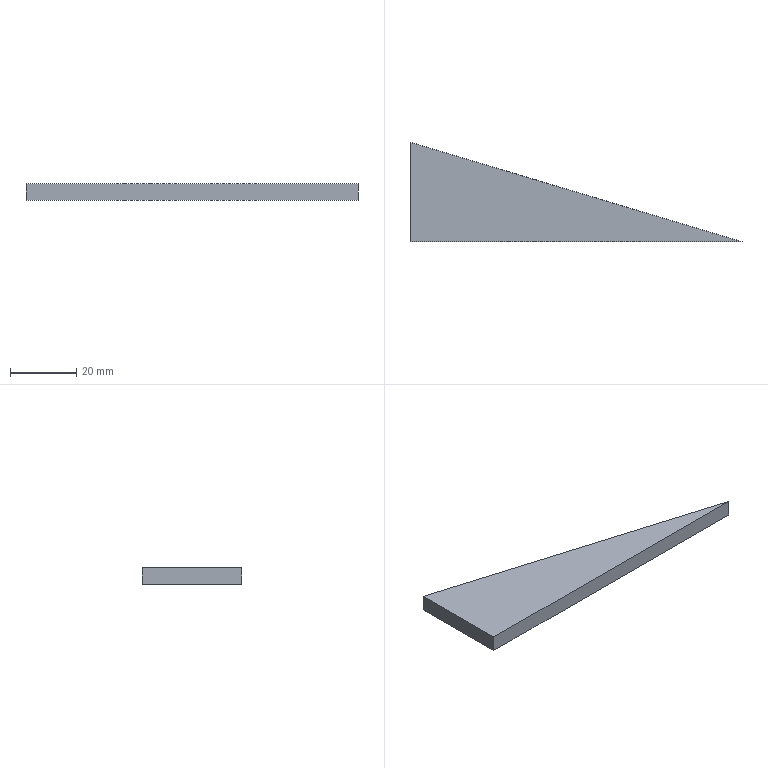Part | SolidWorks | features Extrusion 1 | 1 solid | 5 faces | box 100 x 30 x 5 mm | volume 7500 mm3 | plane 5
STEP:
#1=CARTESIAN_POINT('',(0.,0.,0.));
#2=VERTEX_POINT('',#1);
#3=CARTESIAN_POINT('',(100.,0.,0.));
#4=VERTEX_POINT('',#3);
#5=CARTESIAN_POINT('',(0.,0.,0.));
#6=DIRECTION('',(1.,0.,0.));
#7=VECTOR('',#6,1000.);
#8=LINE('',#5,#7);
#9=EDGE_CURVE('',#2,#4,#8,.T.);
#10=ORIENTED_EDGE('',*,*,#9,.T.);
#11=CARTESIAN_POINT('',(100.,0.,5.));
#12=VERTEX_POINT('',#11);
#13=CARTESIAN_POINT('',(100.,0.,5.));
#14=DIRECTION('',(0.,0.,-1.));
#15=VECTOR('',#14,1000.);
#16=LINE('',#13,#15);
#17=EDGE_CURVE('',#12,#4,#16,.T.);
#18=ORIENTED_EDGE('',*,*,#17,.F.);
#19=CARTESIAN_POINT('',(0.,0.,5.));
#20=VERTEX_POINT('',#19);
#21=CARTESIAN_POINT('',(0.,0.,5.));
#22=DIRECTION('',(1.,0.,0.));
#23=VECTOR('',#22,1000.);
#24=LINE('',#21,#23);
#25=EDGE_CURVE('',#20,#12,#24,.T.);
#26=ORIENTED_EDGE('',*,*,#25,.F.);
#27=CARTESIAN_POINT('',(0.,0.,5.));
#28=DIRECTION('',(0.,0.,-1.));
#29=VECTOR('',#28,1000.);
#30=LINE('',#27,#29);
#31=EDGE_CURVE('',#20,#2,#30,.T.);
#32=ORIENTED_EDGE('',*,*,#31,.T.);
#33=EDGE_LOOP('',(#10,#18,#26,#32));
#34=FACE_OUTER_BOUND('',#33,.T.);
#35=CARTESIAN_POINT('',(0.,0.,5.));
#36=DIRECTION('',(0.,1.,0.));
#37=DIRECTION('',(0.,0.,1.));
#38=AXIS2_PLACEMENT_3D('',#35,#36,#37);
#39=PLANE('',#38);
#40=ADVANCED_FACE('',(#34),#39,.F.);
#41=CARTESIAN_POINT('',(0.,30.,0.));
#42=VERTEX_POINT('',#41);
#43=CARTESIAN_POINT('',(100.,0.,0.));
#44=DIRECTION('',(-0.9578,0.2873,0.));
#45=VECTOR('',#44,1000.);
#46=LINE('',#43,#45);
#47=EDGE_CURVE('',#4,#42,#46,.T.);
#48=ORIENTED_EDGE('',*,*,#47,.T.);
#49=CARTESIAN_POINT('',(0.,30.,5.));
#50=VERTEX_POINT('',#49);
#51=CARTESIAN_POINT('',(0.,30.,5.));
#52=DIRECTION('',(0.,0.,-1.));
#53=VECTOR('',#52,1000.);
#54=LINE('',#51,#53);
#55=EDGE_CURVE('',#50,#42,#54,.T.);
#56=ORIENTED_EDGE('',*,*,#55,.F.);
#57=CARTESIAN_POINT('',(100.,0.,5.));
#58=DIRECTION('',(-0.9578,0.2873,0.));
#59=VECTOR('',#58,1000.);
#60=LINE('',#57,#59);
#61=EDGE_CURVE('',#12,#50,#60,.T.);
#62=ORIENTED_EDGE('',*,*,#61,.F.);
#63=ORIENTED_EDGE('',*,*,#17,.T.);
#64=EDGE_LOOP('',(#48,#56,#62,#63));
#65=FACE_OUTER_BOUND('',#64,.T.);
#66=CARTESIAN_POINT('',(100.,0.,5.));
#67=DIRECTION('',(-0.2873,-0.9578,0.));
#68=DIRECTION('',(0.9578,-0.2873,0.));
#69=AXIS2_PLACEMENT_3D('',#66,#67,#68);
#70=PLANE('',#69);
#71=ADVANCED_FACE('',(#65),#70,.F.);
#72=CARTESIAN_POINT('',(0.,0.,0.));
#73=DIRECTION('',(0.,-1.,0.));
#74=VECTOR('',#73,1000.);
#75=LINE('',#72,#74);
#76=EDGE_CURVE('',#42,#2,#75,.T.);
#77=ORIENTED_EDGE('',*,*,#76,.T.);
#78=ORIENTED_EDGE('',*,*,#31,.F.);
#79=CARTESIAN_POINT('',(0.,0.,5.));
#80=DIRECTION('',(0.,-1.,0.));
#81=VECTOR('',#80,1000.);
#82=LINE('',#79,#81);
#83=EDGE_CURVE('',#50,#20,#82,.T.);
#84=ORIENTED_EDGE('',*,*,#83,.F.);
#85=ORIENTED_EDGE('',*,*,#55,.T.);
#86=EDGE_LOOP('',(#77,#78,#84,#85));
#87=FACE_OUTER_BOUND('',#86,.T.);
#88=CARTESIAN_POINT('',(0.,0.,5.));
#89=DIRECTION('',(1.,0.,0.));
#90=DIRECTION('',(0.,0.,-1.));
#91=AXIS2_PLACEMENT_3D('',#88,#89,#90);
#92=PLANE('',#91);
#93=ADVANCED_FACE('',(#87),#92,.F.);
#94=ORIENTED_EDGE('',*,*,#25,.T.);
#95=ORIENTED_EDGE('',*,*,#61,.T.);
#96=ORIENTED_EDGE('',*,*,#83,.T.);
#97=EDGE_LOOP('',(#94,#95,#96));
#98=FACE_OUTER_BOUND('',#97,.T.);
#99=CARTESIAN_POINT('',(0.,0.,5.));
#100=DIRECTION('',(0.,0.,1.));
#101=DIRECTION('',(1.,0.,0.));
#102=AXIS2_PLACEMENT_3D('',#99,#100,#101);
#103=PLANE('',#102);
#104=ADVANCED_FACE('',(#98),#103,.T.);
#105=ORIENTED_EDGE('',*,*,#9,.F.);
#106=ORIENTED_EDGE('',*,*,#76,.F.);
#107=ORIENTED_EDGE('',*,*,#47,.F.);
#108=EDGE_LOOP('',(#105,#106,#107));
#109=FACE_OUTER_BOUND('',#108,.T.);
#110=CARTESIAN_POINT('',(0.,0.,0.));
#111=DIRECTION('',(0.,0.,1.));
#112=DIRECTION('',(1.,0.,0.));
#113=AXIS2_PLACEMENT_3D('',#110,#111,#112);
#114=PLANE('',#113);
#115=ADVANCED_FACE('',(#109),#114,.F.);
#116=CLOSED_SHELL('',(#40,#71,#93,#104,#115));
#117=MANIFOLD_SOLID_BREP('',#116);
#118=CARTESIAN_POINT('',(0.,0.,0.));
#119=DIRECTION('',(0.,0.,1.));
#120=DIRECTION('',(1.,0.,0.));
#121=AXIS2_PLACEMENT_3D('',#118,#119,#120);
#122=(LENGTH_UNIT()NAMED_UNIT(*)SI_UNIT(.MILLI.,.METRE.));
#123=UNCERTAINTY_MEASURE_WITH_UNIT(LENGTH_MEASURE(0.00001),#122,'','');
#124=(NAMED_UNIT(*)PLANE_ANGLE_UNIT()SI_UNIT($,.RADIAN.));
#125=(NAMED_UNIT(*)SI_UNIT($,.STERADIAN.)SOLID_ANGLE_UNIT());
#126=(GEOMETRIC_REPRESENTATION_CONTEXT(3)GLOBAL_UNCERTAINTY_ASSIGNED_CONTEXT((#123))GLOBAL_UNIT_ASSIGNED_CONTEXT((#122,#124,#125))REPRESENTATION_CONTEXT('',''));
#127=ADVANCED_BREP_SHAPE_REPRESENTATION('',(#117,#121),#126);